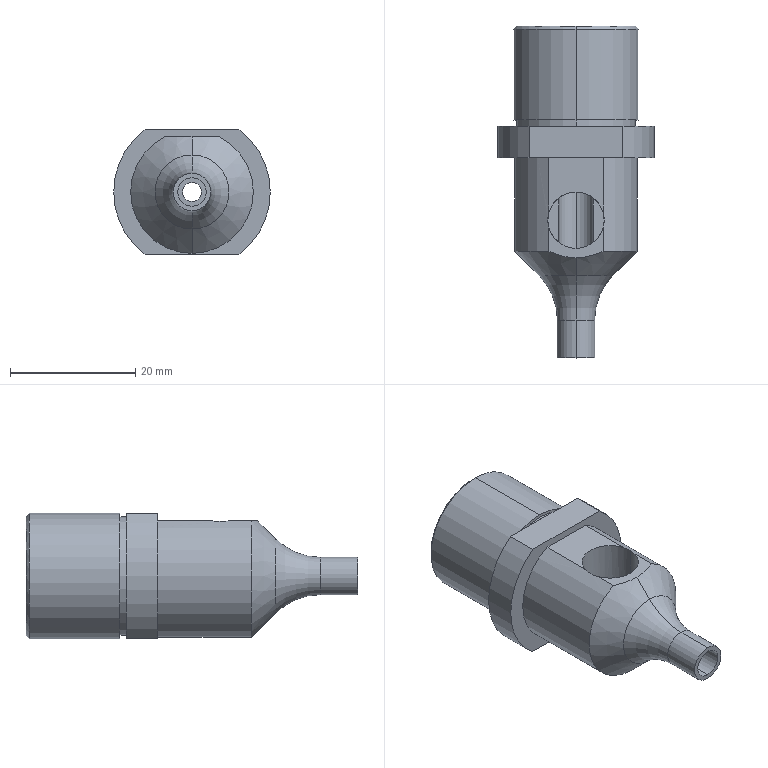Part | SolidWorks | features ICE 7, HoleWzd 4, 3DProfileFeature 2, Chamfer 2, Extrusion 1, Fillet 1, RevCut 1, Revolution 1 | 1 solid | 49 faces | box 25 x 53 x 20 mm | volume 8091 mm3 | cylinder 24 | plane 15 | cone 8 | torus 2 | commonest cylinder face diameters 16 x4 3 x2 4.55 x2 5.5 x2 6 x2 9 x2
STEP:
#1=CARTESIAN_POINT('',(0.,-39.871,-5.929));
#2=VERTEX_POINT('',#1);
#3=CARTESIAN_POINT('',(0.,-39.871,5.929));
#4=VERTEX_POINT('',#3);
#5=CARTESIAN_POINT('',(0.,-39.871,0.));
#6=DIRECTION('',(0.,1.,0.));
#7=DIRECTION('',(0.,0.,-1.));
#8=AXIS2_PLACEMENT_3D('',#5,#6,#7);
#9=CIRCLE('',#8,5.929);
#10=EDGE_CURVE('',#2,#4,#9,.T.);
#11=ORIENTED_EDGE('',*,*,#10,.F.);
#12=CARTESIAN_POINT('',(0.,-46.942,-3.));
#13=VERTEX_POINT('',#12);
#14=CARTESIAN_POINT('',(0.,-46.942,-13.));
#15=DIRECTION('',(1.,0.,0.));
#16=DIRECTION('',(0.,0.,-1.));
#17=AXIS2_PLACEMENT_3D('',#14,#15,#16);
#18=CIRCLE('',#17,10.);
#19=EDGE_CURVE('',#2,#13,#18,.T.);
#20=ORIENTED_EDGE('',*,*,#19,.T.);
#21=CARTESIAN_POINT('',(0.,-46.942,3.));
#22=VERTEX_POINT('',#21);
#23=CARTESIAN_POINT('',(0.,-46.942,0.));
#24=DIRECTION('',(0.,-1.,0.));
#25=DIRECTION('',(0.,0.,1.));
#26=AXIS2_PLACEMENT_3D('',#23,#24,#25);
#27=CIRCLE('',#26,3.);
#28=EDGE_CURVE('',#22,#13,#27,.T.);
#29=ORIENTED_EDGE('',*,*,#28,.F.);
#30=CARTESIAN_POINT('',(0.,-46.942,13.));
#31=DIRECTION('',(-1.,0.,0.));
#32=DIRECTION('',(0.,0.,1.));
#33=AXIS2_PLACEMENT_3D('',#30,#31,#32);
#34=CIRCLE('',#33,10.);
#35=EDGE_CURVE('',#4,#22,#34,.T.);
#36=ORIENTED_EDGE('',*,*,#35,.F.);
#37=EDGE_LOOP('',(#11,#20,#29,#36));
#38=FACE_OUTER_BOUND('',#37,.T.);
#39=CARTESIAN_POINT('',(0.,-46.942,0.));
#40=DIRECTION('',(0.,1.,0.));
#41=DIRECTION('',(0.,0.,1.));
#42=AXIS2_PLACEMENT_3D('',#39,#40,#41);
#43=TOROIDAL_SURFACE('',#42,13.,10.);
#44=ADVANCED_FACE('',(#38),#43,.F.);
#45=CARTESIAN_POINT('',(0.,-48.5,2.275));
#46=VERTEX_POINT('',#45);
#47=CARTESIAN_POINT('',(0.,-48.5,-2.275));
#48=VERTEX_POINT('',#47);
#49=CARTESIAN_POINT('',(0.,-48.5,0.));
#50=DIRECTION('',(0.,-1.,0.));
#51=DIRECTION('',(0.,0.,-1.));
#52=AXIS2_PLACEMENT_3D('',#49,#50,#51);
#53=CIRCLE('',#52,2.275);
#54=EDGE_CURVE('',#46,#48,#53,.T.);
#55=ORIENTED_EDGE('',*,*,#54,.F.);
#56=CARTESIAN_POINT('',(0.,-53.,2.275));
#57=VERTEX_POINT('',#56);
#58=CARTESIAN_POINT('',(0.,-48.5,2.275));
#59=DIRECTION('',(0.,-1.,0.));
#60=VECTOR('',#59,1000.);
#61=LINE('',#58,#60);
#62=EDGE_CURVE('',#46,#57,#61,.T.);
#63=ORIENTED_EDGE('',*,*,#62,.T.);
#64=CARTESIAN_POINT('',(0.,-53.,-2.275));
#65=VERTEX_POINT('',#64);
#66=CARTESIAN_POINT('',(0.,-53.,0.));
#67=DIRECTION('',(0.,-1.,0.));
#68=DIRECTION('',(0.,0.,-1.));
#69=AXIS2_PLACEMENT_3D('',#66,#67,#68);
#70=CIRCLE('',#69,2.275);
#71=EDGE_CURVE('',#57,#65,#70,.T.);
#72=ORIENTED_EDGE('',*,*,#71,.T.);
#73=CARTESIAN_POINT('',(0.,-48.5,-2.275));
#74=DIRECTION('',(0.,-1.,0.));
#75=VECTOR('',#74,1000.);
#76=LINE('',#73,#75);
#77=EDGE_CURVE('',#48,#65,#76,.T.);
#78=ORIENTED_EDGE('',*,*,#77,.F.);
#79=EDGE_LOOP('',(#55,#63,#72,#78));
#80=FACE_OUTER_BOUND('',#79,.T.);
#81=CARTESIAN_POINT('',(0.,-48.5,0.));
#82=DIRECTION('',(0.,-1.,0.));
#83=DIRECTION('',(0.,0.,-1.));
#84=AXIS2_PLACEMENT_3D('',#81,#82,#83);
#85=CYLINDRICAL_SURFACE('',#84,2.275);
#86=ADVANCED_FACE('',(#80),#85,.F.);
#87=CARTESIAN_POINT('',(0.,-43.751,1.5));
#88=VERTEX_POINT('',#87);
#89=CARTESIAN_POINT('',(0.,-43.751,-1.5));
#90=VERTEX_POINT('',#89);
#91=CARTESIAN_POINT('',(0.,-43.751,0.));
#92=DIRECTION('',(0.,-1.,0.));
#93=DIRECTION('',(0.,0.,1.));
#94=AXIS2_PLACEMENT_3D('',#91,#92,#93);
#95=CIRCLE('',#94,1.5);
#96=EDGE_CURVE('',#88,#90,#95,.T.);
#97=ORIENTED_EDGE('',*,*,#96,.T.);
#98=CARTESIAN_POINT('',(0.,-43.,-2.75));
#99=VERTEX_POINT('',#98);
#100=CARTESIAN_POINT('',(0.,-43.,-2.75));
#101=DIRECTION('',(0.,0.515,-0.8572));
#102=VECTOR('',#101,1000.);
#103=LINE('',#100,#102);
#104=EDGE_CURVE('',#90,#99,#103,.T.);
#105=ORIENTED_EDGE('',*,*,#104,.T.);
#106=CARTESIAN_POINT('',(0.,-43.,2.75));
#107=VERTEX_POINT('',#106);
#108=CARTESIAN_POINT('',(0.,-43.,0.));
#109=DIRECTION('',(0.,1.,0.));
#110=DIRECTION('',(0.,0.,1.));
#111=AXIS2_PLACEMENT_3D('',#108,#109,#110);
#112=CIRCLE('',#111,2.75);
#113=EDGE_CURVE('',#99,#107,#112,.T.);
#114=ORIENTED_EDGE('',*,*,#113,.T.);
#115=CARTESIAN_POINT('',(0.,-43.,2.75));
#116=DIRECTION('',(0.,0.515,0.8572));
#117=VECTOR('',#116,1000.);
#118=LINE('',#115,#117);
#119=EDGE_CURVE('',#88,#107,#118,.T.);
#120=ORIENTED_EDGE('',*,*,#119,.F.);
#121=EDGE_LOOP('',(#97,#105,#114,#120));
#122=FACE_OUTER_BOUND('',#121,.T.);
#123=CARTESIAN_POINT('',(0.,-43.,0.));
#124=DIRECTION('',(0.,1.,0.));
#125=DIRECTION('',(0.,0.,1.));
#126=AXIS2_PLACEMENT_3D('',#123,#124,#125);
#127=CONICAL_SURFACE('',#126,2.75,1.03);
#128=ADVANCED_FACE('',(#122),#127,.F.);
#129=ORIENTED_EDGE('',*,*,#113,.F.);
#130=CARTESIAN_POINT('',(0.,-18.,-2.75));
#131=VERTEX_POINT('',#130);
#132=CARTESIAN_POINT('',(0.,-18.,-2.75));
#133=DIRECTION('',(0.,1.,0.));
#134=VECTOR('',#133,1000.);
#135=LINE('',#132,#134);
#136=EDGE_CURVE('',#99,#131,#135,.T.);
#137=ORIENTED_EDGE('',*,*,#136,.T.);
#138=CARTESIAN_POINT('',(0.,-18.,2.75));
#139=VERTEX_POINT('',#138);
#140=CARTESIAN_POINT('',(0.,-18.,0.));
#141=DIRECTION('',(0.,1.,0.));
#142=DIRECTION('',(0.,0.,1.));
#143=AXIS2_PLACEMENT_3D('',#140,#141,#142);
#144=CIRCLE('',#143,2.75);
#145=EDGE_CURVE('',#131,#139,#144,.T.);
#146=ORIENTED_EDGE('',*,*,#145,.T.);
#147=CARTESIAN_POINT('',(0.,-26.5,2.75));
#148=VERTEX_POINT('',#147);
#149=CARTESIAN_POINT('',(0.,-18.,2.75));
#150=DIRECTION('',(0.,1.,0.));
#151=VECTOR('',#150,1000.);
#152=LINE('',#149,#151);
#153=EDGE_CURVE('',#148,#139,#152,.T.);
#154=ORIENTED_EDGE('',*,*,#153,.F.);
#155=CARTESIAN_POINT('',(-2.75,-27.438,0.));
#156=VERTEX_POINT('',#155);
#157=CARTESIAN_POINT('',(-2.75,-27.438,0.));
#158=CARTESIAN_POINT('',(-2.75,-27.438,0.1874));
#159=CARTESIAN_POINT('',(-2.731,-27.423,0.3702));
#160=CARTESIAN_POINT('',(-2.658,-27.369,0.7279));
#161=CARTESIAN_POINT('',(-2.603,-27.329,0.904));
#162=CARTESIAN_POINT('',(-2.395,-27.186,1.398));
#163=CARTESIAN_POINT('',(-2.194,-27.062,1.694));
#164=CARTESIAN_POINT('',(-1.823,-26.884,2.066));
#165=CARTESIAN_POINT('',(-1.686,-26.825,2.18));
#166=CARTESIAN_POINT('',(-1.392,-26.718,2.378));
#167=CARTESIAN_POINT('',(-1.237,-26.67,2.463));
#168=CARTESIAN_POINT('',(-0.9051,-26.589,2.603));
#169=CARTESIAN_POINT('',(-0.7273,-26.555,2.658));
#170=CARTESIAN_POINT('',(-0.3687,-26.511,2.731));
#171=CARTESIAN_POINT('',(-0.1861,-26.5,2.75));
#172=CARTESIAN_POINT('',(0.,-26.5,2.75));
#173=B_SPLINE_CURVE_WITH_KNOTS('',3,(#157,#158,#159,#160,#161,#162,#163,#164,#165,#166,#167,#168,#169,#170,#171,#172),.UNSPECIFIED.,.F.,.F.,(4,2,2,2,2,2,2,4),(0.,0.0005525,0.001105,0.00221,0.002762,0.003315,0.003867,0.00442),.UNSPECIFIED.);
#174=EDGE_CURVE('',#156,#148,#173,.T.);
#175=ORIENTED_EDGE('',*,*,#174,.F.);
#176=CARTESIAN_POINT('',(-2.75,-34.562,0.));
#177=VERTEX_POINT('',#176);
#178=CARTESIAN_POINT('',(-2.75,-18.,0.));
#179=DIRECTION('',(0.,1.,0.));
#180=VECTOR('',#179,1000.);
#181=LINE('',#178,#180);
#182=EDGE_CURVE('',#177,#156,#181,.T.);
#183=ORIENTED_EDGE('',*,*,#182,.F.);
#184=CARTESIAN_POINT('',(0.,-35.5,2.75));
#185=VERTEX_POINT('',#184);
#186=CARTESIAN_POINT('',(0.,-35.5,2.75));
#187=CARTESIAN_POINT('',(-0.1857,-35.5,2.75));
#188=CARTESIAN_POINT('',(-0.3713,-35.488,2.731));
#189=CARTESIAN_POINT('',(-0.7299,-35.444,2.658));
#190=CARTESIAN_POINT('',(-0.9067,-35.411,2.602));
#191=CARTESIAN_POINT('',(-1.405,-35.289,2.391));
#192=CARTESIAN_POINT('',(-1.703,-35.174,2.187));
#193=CARTESIAN_POINT('',(-2.073,-34.997,1.816));
#194=CARTESIAN_POINT('',(-2.185,-34.935,1.679));
#195=CARTESIAN_POINT('',(-2.381,-34.82,1.387));
#196=CARTESIAN_POINT('',(-2.465,-34.766,1.232));
#197=CARTESIAN_POINT('',(-2.603,-34.672,0.9044));
#198=CARTESIAN_POINT('',(-2.658,-34.631,0.7283));
#199=CARTESIAN_POINT('',(-2.731,-34.577,0.3702));
#200=CARTESIAN_POINT('',(-2.75,-34.562,0.1873));
#201=CARTESIAN_POINT('',(-2.75,-34.562,0.));
#202=B_SPLINE_CURVE_WITH_KNOTS('',3,(#186,#187,#188,#189,#190,#191,#192,#193,#194,#195,#196,#197,#198,#199,#200,#201),.UNSPECIFIED.,.F.,.F.,(4,2,2,2,2,2,2,4),(0.00442,0.004971,0.005522,0.006624,0.007176,0.007727,0.008278,0.008829),.UNSPECIFIED.);
#203=EDGE_CURVE('',#185,#177,#202,.T.);
#204=ORIENTED_EDGE('',*,*,#203,.F.);
#205=CARTESIAN_POINT('',(0.,-18.,2.75));
#206=DIRECTION('',(0.,1.,0.));
#207=VECTOR('',#206,1000.);
#208=LINE('',#205,#207);
#209=EDGE_CURVE('',#107,#185,#208,.T.);
#210=ORIENTED_EDGE('',*,*,#209,.F.);
#211=EDGE_LOOP('',(#129,#137,#146,#154,#175,#183,#204,#210));
#212=FACE_OUTER_BOUND('',#211,.T.);
#213=CARTESIAN_POINT('',(0.,-18.,0.));
#214=DIRECTION('',(0.,1.,0.));
#215=DIRECTION('',(0.,0.,1.));
#216=AXIS2_PLACEMENT_3D('',#213,#214,#215);
#217=CYLINDRICAL_SURFACE('',#216,2.75);
#218=ADVANCED_FACE('',(#212),#217,.F.);
#219=CARTESIAN_POINT('',(0.,-53.,3.));
#220=VERTEX_POINT('',#219);
#221=CARTESIAN_POINT('',(0.,-53.,-3.));
#222=VERTEX_POINT('',#221);
#223=CARTESIAN_POINT('',(0.,-53.,0.));
#224=DIRECTION('',(0.,1.,0.));
#225=DIRECTION('',(0.,0.,1.));
#226=AXIS2_PLACEMENT_3D('',#223,#224,#225);
#227=CIRCLE('',#226,3.);
#228=EDGE_CURVE('',#220,#222,#227,.T.);
#229=ORIENTED_EDGE('',*,*,#228,.T.);
#230=CARTESIAN_POINT('',(0.,2.516,-3.));
#231=DIRECTION('',(0.,1.,0.));
#232=VECTOR('',#231,1000.);
#233=LINE('',#230,#232);
#234=EDGE_CURVE('',#222,#13,#233,.T.);
#235=ORIENTED_EDGE('',*,*,#234,.T.);
#236=CARTESIAN_POINT('',(0.,-46.942,0.));
#237=DIRECTION('',(0.,-1.,0.));
#238=DIRECTION('',(0.,0.,1.));
#239=AXIS2_PLACEMENT_3D('',#236,#237,#238);
#240=CIRCLE('',#239,3.);
#241=EDGE_CURVE('',#13,#22,#240,.T.);
#242=ORIENTED_EDGE('',*,*,#241,.T.);
#243=CARTESIAN_POINT('',(0.,2.516,3.));
#244=DIRECTION('',(0.,1.,0.));
#245=VECTOR('',#244,1000.);
#246=LINE('',#243,#245);
#247=EDGE_CURVE('',#220,#22,#246,.T.);
#248=ORIENTED_EDGE('',*,*,#247,.F.);
#249=EDGE_LOOP('',(#229,#235,#242,#248));
#250=FACE_OUTER_BOUND('',#249,.T.);
#251=CARTESIAN_POINT('',(0.,2.516,0.));
#252=DIRECTION('',(0.,1.,0.));
#253=DIRECTION('',(0.,0.,1.));
#254=AXIS2_PLACEMENT_3D('',#251,#252,#253);
#255=CYLINDRICAL_SURFACE('',#254,3.);
#256=ADVANCED_FACE('',(#250),#255,.T.);
#257=CARTESIAN_POINT('',(0.,-39.871,0.));
#258=DIRECTION('',(0.,1.,0.));
#259=DIRECTION('',(0.,0.,-1.));
#260=AXIS2_PLACEMENT_3D('',#257,#258,#259);
#261=CIRCLE('',#260,5.929);
#262=EDGE_CURVE('',#4,#2,#261,.T.);
#263=ORIENTED_EDGE('',*,*,#262,.T.);
#264=CARTESIAN_POINT('',(0.,-36.,-9.8));
#265=VERTEX_POINT('',#264);
#266=CARTESIAN_POINT('',(0.,-38.,-7.8));
#267=DIRECTION('',(0.,0.7071,-0.7071));
#268=VECTOR('',#267,1000.);
#269=LINE('',#266,#268);
#270=EDGE_CURVE('',#2,#265,#269,.T.);
#271=ORIENTED_EDGE('',*,*,#270,.T.);
#272=CARTESIAN_POINT('',(4.313,-36.,8.8));
#273=VERTEX_POINT('',#272);
#274=CARTESIAN_POINT('',(0.,-36.,0.));
#275=DIRECTION('',(0.,1.,0.));
#276=DIRECTION('',(0.,0.,1.));
#277=AXIS2_PLACEMENT_3D('',#274,#275,#276);
#278=CIRCLE('',#277,9.8);
#279=EDGE_CURVE('',#273,#265,#278,.T.);
#280=ORIENTED_EDGE('',*,*,#279,.F.);
#281=CARTESIAN_POINT('',(0.,-37.,8.8));
#282=VERTEX_POINT('',#281);
#283=CARTESIAN_POINT('',(0.,-37.,8.8));
#284=CARTESIAN_POINT('',(0.7477,-37.,8.8));
#285=CARTESIAN_POINT('',(1.48,-36.904,8.8));
#286=CARTESIAN_POINT('',(2.921,-36.554,8.8));
#287=CARTESIAN_POINT('',(3.634,-36.299,8.8));
#288=CARTESIAN_POINT('',(4.313,-36.,8.8));
#289=B_SPLINE_CURVE_WITH_KNOTS('',3,(#283,#284,#285,#286,#287,#288),.UNSPECIFIED.,.F.,.F.,(4,2,4),(0.00443,0.006647,0.008864),.UNSPECIFIED.);
#290=EDGE_CURVE('',#282,#273,#289,.T.);
#291=ORIENTED_EDGE('',*,*,#290,.F.);
#292=CARTESIAN_POINT('',(0.,-38.,7.8));
#293=DIRECTION('',(0.,0.7071,0.7071));
#294=VECTOR('',#293,1000.);
#295=LINE('',#292,#294);
#296=EDGE_CURVE('',#4,#282,#295,.T.);
#297=ORIENTED_EDGE('',*,*,#296,.F.);
#298=EDGE_LOOP('',(#263,#271,#280,#291,#297));
#299=FACE_OUTER_BOUND('',#298,.T.);
#300=CARTESIAN_POINT('',(0.,-38.,0.));
#301=DIRECTION('',(0.,1.,0.));
#302=DIRECTION('',(0.,0.,1.));
#303=AXIS2_PLACEMENT_3D('',#300,#301,#302);
#304=CONICAL_SURFACE('',#303,7.8,0.7854);
#305=ADVANCED_FACE('',(#299),#304,.T.);
#306=CARTESIAN_POINT('',(0.,-15.,9.5));
#307=VERTEX_POINT('',#306);
#308=CARTESIAN_POINT('',(0.,-15.,-9.5));
#309=VERTEX_POINT('',#308);
#310=CARTESIAN_POINT('',(0.,-15.,0.));
#311=DIRECTION('',(0.,1.,0.));
#312=DIRECTION('',(0.,0.,1.));
#313=AXIS2_PLACEMENT_3D('',#310,#311,#312);
#314=CIRCLE('',#313,9.5);
#315=EDGE_CURVE('',#307,#309,#314,.T.);
#316=ORIENTED_EDGE('',*,*,#315,.F.);
#317=CARTESIAN_POINT('',(0.,-16.,9.5));
#318=VERTEX_POINT('',#317);
#319=CARTESIAN_POINT('',(0.,-15.,9.5));
#320=DIRECTION('',(0.,-1.,0.));
#321=VECTOR('',#320,1000.);
#322=LINE('',#319,#321);
#323=EDGE_CURVE('',#307,#318,#322,.T.);
#324=ORIENTED_EDGE('',*,*,#323,.T.);
#325=CARTESIAN_POINT('',(0.,-16.,-9.5));
#326=VERTEX_POINT('',#325);
#327=CARTESIAN_POINT('',(0.,-16.,0.));
#328=DIRECTION('',(0.,1.,0.));
#329=DIRECTION('',(0.,0.,1.));
#330=AXIS2_PLACEMENT_3D('',#327,#328,#329);
#331=CIRCLE('',#330,9.5);
#332=EDGE_CURVE('',#318,#326,#331,.T.);
#333=ORIENTED_EDGE('',*,*,#332,.T.);
#334=CARTESIAN_POINT('',(0.,-15.,-9.5));
#335=DIRECTION('',(0.,-1.,0.));
#336=VECTOR('',#335,1000.);
#337=LINE('',#334,#336);
#338=EDGE_CURVE('',#309,#326,#337,.T.);
#339=ORIENTED_EDGE('',*,*,#338,.F.);
#340=EDGE_LOOP('',(#316,#324,#333,#339));
#341=FACE_OUTER_BOUND('',#340,.T.);
#342=CARTESIAN_POINT('',(0.,-15.,0.));
#343=DIRECTION('',(0.,-1.,0.));
#344=DIRECTION('',(0.,0.,-1.));
#345=AXIS2_PLACEMENT_3D('',#342,#343,#344);
#346=CYLINDRICAL_SURFACE('',#345,9.5);
#347=ADVANCED_FACE('',(#341),#346,.T.);
#348=CARTESIAN_POINT('',(0.,-0.5,-8.));
#349=VERTEX_POINT('',#348);
#350=CARTESIAN_POINT('',(0.,-0.5,8.));
#351=VERTEX_POINT('',#350);
#352=CARTESIAN_POINT('',(0.,-0.5,0.));
#353=DIRECTION('',(0.,1.,0.));
#354=DIRECTION('',(0.,0.,1.));
#355=AXIS2_PLACEMENT_3D('',#352,#353,#354);
#356=CIRCLE('',#355,8.);
#357=EDGE_CURVE('',#349,#351,#356,.T.);
#358=ORIENTED_EDGE('',*,*,#357,.F.);
#359=CARTESIAN_POINT('',(0.,0.,-8.5));
#360=VERTEX_POINT('',#359);
#361=CARTESIAN_POINT('',(0.,-0.5,-8.));
#362=DIRECTION('',(0.,0.7071,-0.7071));
#363=VECTOR('',#362,1000.);
#364=LINE('',#361,#363);
#365=EDGE_CURVE('',#349,#360,#364,.T.);
#366=ORIENTED_EDGE('',*,*,#365,.T.);
#367=CARTESIAN_POINT('',(0.,0.,8.5));
#368=VERTEX_POINT('',#367);
#369=CARTESIAN_POINT('',(0.,0.,0.));
#370=DIRECTION('',(0.,-1.,0.));
#371=DIRECTION('',(0.,0.,1.));
#372=AXIS2_PLACEMENT_3D('',#369,#370,#371);
#373=CIRCLE('',#372,8.5);
#374=EDGE_CURVE('',#368,#360,#373,.T.);
#375=ORIENTED_EDGE('',*,*,#374,.F.);
#376=CARTESIAN_POINT('',(0.,-0.5,8.));
#377=DIRECTION('',(0.,0.7071,0.7071));
#378=VECTOR('',#377,1000.);
#379=LINE('',#376,#378);
#380=EDGE_CURVE('',#351,#368,#379,.T.);
#381=ORIENTED_EDGE('',*,*,#380,.F.);
#382=EDGE_LOOP('',(#358,#366,#375,#381));
#383=FACE_OUTER_BOUND('',#382,.T.);
#384=CARTESIAN_POINT('',(0.,-0.5,0.));
#385=DIRECTION('',(0.,1.,0.));
#386=DIRECTION('',(0.,0.,1.));
#387=AXIS2_PLACEMENT_3D('',#384,#385,#386);
#388=CONICAL_SURFACE('',#387,8.,0.7854);
#389=ADVANCED_FACE('',(#383),#388,.F.);
#390=CARTESIAN_POINT('',(0.,0.,9.5));
#391=VERTEX_POINT('',#390);
#392=CARTESIAN_POINT('',(0.,0.,-9.5));
#393=VERTEX_POINT('',#392);
#394=CARTESIAN_POINT('',(0.,0.,0.));
#395=DIRECTION('',(0.,1.,0.));
#396=DIRECTION('',(0.,0.,1.));
#397=AXIS2_PLACEMENT_3D('',#394,#395,#396);
#398=CIRCLE('',#397,9.5);
#399=EDGE_CURVE('',#391,#393,#398,.T.);
#400=ORIENTED_EDGE('',*,*,#399,.F.);
#401=CARTESIAN_POINT('',(0.,-0.5,10.));
#402=VERTEX_POINT('',#401);
#403=CARTESIAN_POINT('',(0.,0.,9.5));
#404=DIRECTION('',(0.,-0.7071,0.7071));
#405=VECTOR('',#404,1000.);
#406=LINE('',#403,#405);
#407=EDGE_CURVE('',#391,#402,#406,.T.);
#408=ORIENTED_EDGE('',*,*,#407,.T.);
#409=CARTESIAN_POINT('',(0.,-0.5,-10.));
#410=VERTEX_POINT('',#409);
#411=CARTESIAN_POINT('',(0.,-0.5,0.));
#412=DIRECTION('',(0.,-1.,0.));
#413=DIRECTION('',(0.,0.,1.));
#414=AXIS2_PLACEMENT_3D('',#411,#412,#413);
#415=CIRCLE('',#414,10.);
#416=EDGE_CURVE('',#410,#402,#415,.T.);
#417=ORIENTED_EDGE('',*,*,#416,.F.);
#418=CARTESIAN_POINT('',(0.,0.,-9.5));
#419=DIRECTION('',(0.,-0.7071,-0.7071));
#420=VECTOR('',#419,1000.);
#421=LINE('',#418,#420);
#422=EDGE_CURVE('',#393,#410,#421,.T.);
#423=ORIENTED_EDGE('',*,*,#422,.F.);
#424=EDGE_LOOP('',(#400,#408,#417,#423));
#425=FACE_OUTER_BOUND('',#424,.T.);
#426=CARTESIAN_POINT('',(0.,0.,0.));
#427=DIRECTION('',(0.,-1.,0.));
#428=DIRECTION('',(0.,0.,-1.));
#429=AXIS2_PLACEMENT_3D('',#426,#427,#428);
#430=CONICAL_SURFACE('',#429,9.5,0.7854);
#431=ADVANCED_FACE('',(#425),#430,.T.);
#432=CARTESIAN_POINT('',(-4.313,-21.,8.8));
#433=VERTEX_POINT('',#432);
#434=CARTESIAN_POINT('',(0.,-21.,-9.8));
#435=VERTEX_POINT('',#434);
#436=CARTESIAN_POINT('',(0.,-21.,0.));
#437=DIRECTION('',(0.,-1.,0.));
#438=DIRECTION('',(0.,0.,1.));
#439=AXIS2_PLACEMENT_3D('',#436,#437,#438);
#440=CIRCLE('',#439,9.8);
#441=EDGE_CURVE('',#433,#435,#440,.T.);
#442=ORIENTED_EDGE('',*,*,#441,.T.);
#443=CARTESIAN_POINT('',(0.,7.284,-9.8));
#444=DIRECTION('',(0.,-1.,0.));
#445=VECTOR('',#444,1000.);
#446=LINE('',#443,#445);
#447=EDGE_CURVE('',#435,#265,#446,.T.);
#448=ORIENTED_EDGE('',*,*,#447,.T.);
#449=CARTESIAN_POINT('',(-4.313,-36.,8.8));
#450=VERTEX_POINT('',#449);
#451=CARTESIAN_POINT('',(0.,-36.,0.));
#452=DIRECTION('',(0.,1.,0.));
#453=DIRECTION('',(0.,0.,1.));
#454=AXIS2_PLACEMENT_3D('',#451,#452,#453);
#455=CIRCLE('',#454,9.8);
#456=EDGE_CURVE('',#265,#450,#455,.T.);
#457=ORIENTED_EDGE('',*,*,#456,.T.);
#458=CARTESIAN_POINT('',(-4.313,-32.285,8.8));
#459=VERTEX_POINT('',#458);
#460=CARTESIAN_POINT('',(-4.313,7.284,8.8));
#461=DIRECTION('',(0.,-1.,0.));
#462=VECTOR('',#461,1000.);
#463=LINE('',#460,#462);
#464=EDGE_CURVE('',#459,#450,#463,.T.);
#465=ORIENTED_EDGE('',*,*,#464,.F.);
#466=CARTESIAN_POINT('',(-4.5,-31.,8.706));
#467=VERTEX_POINT('',#466);
#468=CARTESIAN_POINT('',(-4.313,-32.285,8.8));
#469=CARTESIAN_POINT('',(-4.374,-32.08,8.77));
#470=CARTESIAN_POINT('',(-4.42,-31.87,8.746));
#471=CARTESIAN_POINT('',(-4.484,-31.44,8.714));
#472=CARTESIAN_POINT('',(-4.5,-31.22,8.706));
#473=CARTESIAN_POINT('',(-4.5,-31.,8.706));
#474=B_SPLINE_CURVE_WITH_KNOTS('',3,(#468,#469,#470,#471,#472,#473),.UNSPECIFIED.,.F.,.F.,(4,2,4),(0.02723,0.02788,0.02852),.UNSPECIFIED.);
#475=EDGE_CURVE('',#459,#467,#474,.T.);
#476=ORIENTED_EDGE('',*,*,#475,.T.);
#477=CARTESIAN_POINT('',(-4.313,-29.715,8.8));
#478=VERTEX_POINT('',#477);
#479=CARTESIAN_POINT('',(-4.5,-31.,8.706));
#480=CARTESIAN_POINT('',(-4.5,-30.78,8.706));
#481=CARTESIAN_POINT('',(-4.484,-30.563,8.714));
#482=CARTESIAN_POINT('',(-4.421,-30.135,8.746));
#483=CARTESIAN_POINT('',(-4.375,-29.923,8.77));
#484=CARTESIAN_POINT('',(-4.313,-29.715,8.8));
#485=B_SPLINE_CURVE_WITH_KNOTS('',3,(#479,#480,#481,#482,#483,#484),.UNSPECIFIED.,.F.,.F.,(4,2,4),(0.,0.0006507,0.001301),.UNSPECIFIED.);
#486=EDGE_CURVE('',#467,#478,#485,.T.);
#487=ORIENTED_EDGE('',*,*,#486,.T.);
#488=CARTESIAN_POINT('',(-4.313,7.284,8.8));
#489=DIRECTION('',(0.,-1.,0.));
#490=VECTOR('',#489,1000.);
#491=LINE('',#488,#490);
#492=EDGE_CURVE('',#433,#478,#491,.T.);
#493=ORIENTED_EDGE('',*,*,#492,.F.);
#494=EDGE_LOOP('',(#442,#448,#457,#465,#476,#487,#493));
#495=FACE_OUTER_BOUND('',#494,.T.);
#496=CARTESIAN_POINT('',(0.,7.284,0.));
#497=DIRECTION('',(0.,-1.,0.));
#498=DIRECTION('',(0.,0.,-1.));
#499=AXIS2_PLACEMENT_3D('',#496,#497,#498);
#500=CYLINDRICAL_SURFACE('',#499,9.8);
#501=ADVANCED_FACE('',(#495),#500,.T.);
#502=CARTESIAN_POINT('',(0.,-1.8,8.5));
#503=VERTEX_POINT('',#502);
#504=CARTESIAN_POINT('',(0.,-1.8,-8.5));
#505=VERTEX_POINT('',#504);
#506=CARTESIAN_POINT('',(0.,-1.8,0.));
#507=DIRECTION('',(0.,-1.,0.));
#508=DIRECTION('',(0.,0.,-1.));
#509=AXIS2_PLACEMENT_3D('',#506,#507,#508);
#510=CIRCLE('',#509,8.5);
#511=EDGE_CURVE('',#503,#505,#510,.T.);
#512=ORIENTED_EDGE('',*,*,#511,.F.);
#513=CARTESIAN_POINT('',(0.,-3.,8.5));
#514=VERTEX_POINT('',#513);
#515=CARTESIAN_POINT('',(0.,-38.,8.5));
#516=DIRECTION('',(0.,-1.,0.));
#517=VECTOR('',#516,1000.);
#518=LINE('',#515,#517);
#519=EDGE_CURVE('',#503,#514,#518,.T.);
#520=ORIENTED_EDGE('',*,*,#519,.T.);
#521=CARTESIAN_POINT('',(0.,-3.,-8.5));
#522=VERTEX_POINT('',#521);
#523=CARTESIAN_POINT('',(0.,-3.,0.));
#524=DIRECTION('',(0.,-1.,0.));
#525=DIRECTION('',(0.,0.,-1.));
#526=AXIS2_PLACEMENT_3D('',#523,#524,#525);
#527=CIRCLE('',#526,8.5);
#528=EDGE_CURVE('',#514,#522,#527,.T.);
#529=ORIENTED_EDGE('',*,*,#528,.T.);
#530=CARTESIAN_POINT('',(0.,-38.,-8.5));
#531=DIRECTION('',(0.,-1.,0.));
#532=VECTOR('',#531,1000.);
#533=LINE('',#530,#532);
#534=EDGE_CURVE('',#505,#522,#533,.T.);
#535=ORIENTED_EDGE('',*,*,#534,.F.);
#536=EDGE_LOOP('',(#512,#520,#529,#535));
#537=FACE_OUTER_BOUND('',#536,.T.);
#538=CARTESIAN_POINT('',(0.,-38.,0.));
#539=DIRECTION('',(0.,-1.,0.));
#540=DIRECTION('',(0.,0.,-1.));
#541=AXIS2_PLACEMENT_3D('',#538,#539,#540);
#542=CYLINDRICAL_SURFACE('',#541,8.5);
#543=ADVANCED_FACE('',(#537),#542,.F.);
#544=CARTESIAN_POINT('',(0.,-18.,-8.));
#545=VERTEX_POINT('',#544);
#546=CARTESIAN_POINT('',(0.,-18.,8.));
#547=VERTEX_POINT('',#546);
#548=CARTESIAN_POINT('',(0.,-18.,0.));
#549=DIRECTION('',(0.,1.,0.));
#550=DIRECTION('',(0.,0.,1.));
#551=AXIS2_PLACEMENT_3D('',#548,#549,#550);
#552=CIRCLE('',#551,8.);
#553=EDGE_CURVE('',#545,#547,#552,.T.);
#554=ORIENTED_EDGE('',*,*,#553,.F.);
#555=CARTESIAN_POINT('',(0.,-3.,-8.));
#556=VERTEX_POINT('',#555);
#557=CARTESIAN_POINT('',(0.,-18.,-8.));
#558=DIRECTION('',(0.,1.,0.));
#559=VECTOR('',#558,1000.);
#560=LINE('',#557,#559);
#561=EDGE_CURVE('',#545,#556,#560,.T.);
#562=ORIENTED_EDGE('',*,*,#561,.T.);
#563=CARTESIAN_POINT('',(0.,-3.,8.));
#564=VERTEX_POINT('',#563);
#565=CARTESIAN_POINT('',(0.,-3.,0.));
#566=DIRECTION('',(0.,1.,0.));
#567=DIRECTION('',(0.,0.,-1.));
#568=AXIS2_PLACEMENT_3D('',#565,#566,#567);
#569=CIRCLE('',#568,8.);
#570=EDGE_CURVE('',#556,#564,#569,.T.);
#571=ORIENTED_EDGE('',*,*,#570,.T.);
#572=CARTESIAN_POINT('',(0.,-18.,8.));
#573=DIRECTION('',(0.,1.,0.));
#574=VECTOR('',#573,1000.);
#575=LINE('',#572,#574);
#576=EDGE_CURVE('',#547,#564,#575,.T.);
#577=ORIENTED_EDGE('',*,*,#576,.F.);
#578=EDGE_LOOP('',(#554,#562,#571,#577));
#579=FACE_OUTER_BOUND('',#578,.T.);
#580=CARTESIAN_POINT('',(0.,-18.,0.));
#581=DIRECTION('',(0.,1.,0.));
#582=DIRECTION('',(0.,0.,1.));
#583=AXIS2_PLACEMENT_3D('',#580,#581,#582);
#584=CYLINDRICAL_SURFACE('',#583,8.);
#585=ADVANCED_FACE('',(#579),#584,.F.);
#586=CARTESIAN_POINT('',(0.,-15.,-10.));
#587=VERTEX_POINT('',#586);
#588=CARTESIAN_POINT('',(0.,-15.,10.));
#589=VERTEX_POINT('',#588);
#590=CARTESIAN_POINT('',(0.,-15.,0.));
#591=DIRECTION('',(0.,-1.,0.));
#592=DIRECTION('',(0.,0.,1.));
#593=AXIS2_PLACEMENT_3D('',#590,#591,#592);
#594=CIRCLE('',#593,10.);
#595=EDGE_CURVE('',#587,#589,#594,.T.);
#596=ORIENTED_EDGE('',*,*,#595,.F.);
#597=CARTESIAN_POINT('',(0.,-38.,-10.));
#598=DIRECTION('',(0.,1.,0.));
#599=VECTOR('',#598,1000.);
#600=LINE('',#597,#599);
#601=EDGE_CURVE('',#587,#410,#600,.T.);
#602=ORIENTED_EDGE('',*,*,#601,.T.);
#603=ORIENTED_EDGE('',*,*,#416,.T.);
#604=CARTESIAN_POINT('',(0.,-38.,10.));
#605=DIRECTION('',(0.,1.,0.));
#606=VECTOR('',#605,1000.);
#607=LINE('',#604,#606);
#608=EDGE_CURVE('',#589,#402,#607,.T.);
#609=ORIENTED_EDGE('',*,*,#608,.F.);
#610=EDGE_LOOP('',(#596,#602,#603,#609));
#611=FACE_OUTER_BOUND('',#610,.T.);
#612=CARTESIAN_POINT('',(0.,-38.,0.));
#613=DIRECTION('',(0.,1.,0.));
#614=DIRECTION('',(0.,0.,1.));
#615=AXIS2_PLACEMENT_3D('',#612,#613,#614);
#616=CYLINDRICAL_SURFACE('',#615,10.);
#617=ADVANCED_FACE('',(#611),#616,.T.);
#618=CARTESIAN_POINT('',(0.,-1.8,8.));
#619=VERTEX_POINT('',#618);
#620=CARTESIAN_POINT('',(0.,-1.8,-8.));
#621=VERTEX_POINT('',#620);
#622=CARTESIAN_POINT('',(0.,-1.8,0.));
#623=DIRECTION('',(0.,-1.,0.));
#624=DIRECTION('',(0.,0.,1.));
#625=AXIS2_PLACEMENT_3D('',#622,#623,#624);
#626=CIRCLE('',#625,8.);
#627=EDGE_CURVE('',#619,#621,#626,.T.);
#628=ORIENTED_EDGE('',*,*,#627,.T.);
#629=CARTESIAN_POINT('',(0.,-18.,-8.));
#630=DIRECTION('',(0.,1.,0.));
#631=VECTOR('',#630,1000.);
#632=LINE('',#629,#631);
#633=EDGE_CURVE('',#621,#349,#632,.T.);
#634=ORIENTED_EDGE('',*,*,#633,.T.);
#635=ORIENTED_EDGE('',*,*,#357,.T.);
#636=CARTESIAN_POINT('',(0.,-18.,8.));
#637=DIRECTION('',(0.,1.,0.));
#638=VECTOR('',#637,1000.);
#639=LINE('',#636,#638);
#640=EDGE_CURVE('',#619,#351,#639,.T.);
#641=ORIENTED_EDGE('',*,*,#640,.F.);
#642=EDGE_LOOP('',(#628,#634,#635,#641));
#643=FACE_OUTER_BOUND('',#642,.T.);
#644=CARTESIAN_POINT('',(0.,-18.,0.));
#645=DIRECTION('',(0.,1.,0.));
#646=DIRECTION('',(0.,0.,1.));
#647=AXIS2_PLACEMENT_3D('',#644,#645,#646);
#648=CYLINDRICAL_SURFACE('',#647,8.);
#649=ADVANCED_FACE('',(#643),#648,.F.);
#650=CARTESIAN_POINT('',(4.5,-31.,8.706));
#651=VERTEX_POINT('',#650);
#652=CARTESIAN_POINT('',(4.313,-32.285,8.8));
#653=VERTEX_POINT('',#652);
#654=CARTESIAN_POINT('',(4.5,-31.,8.706));
#655=CARTESIAN_POINT('',(4.5,-31.216,8.706));
#656=CARTESIAN_POINT('',(4.484,-31.435,8.714));
#657=CARTESIAN_POINT('',(4.421,-31.868,8.746));
#658=CARTESIAN_POINT('',(4.374,-32.079,8.77));
#659=CARTESIAN_POINT('',(4.313,-32.285,8.8));
#660=B_SPLINE_CURVE_WITH_KNOTS('',3,(#654,#655,#656,#657,#658,#659),.UNSPECIFIED.,.F.,.F.,(4,2,4),(0.01427,0.01492,0.01557),.UNSPECIFIED.);
#661=EDGE_CURVE('',#651,#653,#660,.T.);
#662=ORIENTED_EDGE('',*,*,#661,.F.);
#663=CARTESIAN_POINT('',(4.5,-31.,0.));
#664=VERTEX_POINT('',#663);
#665=CARTESIAN_POINT('',(4.5,-31.,0.));
#666=DIRECTION('',(0.,0.,-1.));
#667=VECTOR('',#666,1000.);
#668=LINE('',#665,#667);
#669=EDGE_CURVE('',#651,#664,#668,.T.);
#670=ORIENTED_EDGE('',*,*,#669,.T.);
#671=CARTESIAN_POINT('',(2.75,-34.562,0.));
#672=VERTEX_POINT('',#671);
#673=CARTESIAN_POINT('',(0.,-31.,0.));
#674=DIRECTION('',(0.,0.,-1.));
#675=DIRECTION('',(-1.,0.,0.));
#676=AXIS2_PLACEMENT_3D('',#673,#674,#675);
#677=CIRCLE('',#676,4.5);
#678=EDGE_CURVE('',#664,#672,#677,.T.);
#679=ORIENTED_EDGE('',*,*,#678,.T.);
#680=CARTESIAN_POINT('',(2.75,-34.562,0.));
#681=CARTESIAN_POINT('',(2.75,-34.562,0.1874));
#682=CARTESIAN_POINT('',(2.731,-34.577,0.3702));
#683=CARTESIAN_POINT('',(2.658,-34.631,0.7279));
#684=CARTESIAN_POINT('',(2.603,-34.671,0.904));
#685=CARTESIAN_POINT('',(2.395,-34.814,1.398));
#686=CARTESIAN_POINT('',(2.194,-34.938,1.694));
#687=CARTESIAN_POINT('',(1.823,-35.116,2.066));
#688=CARTESIAN_POINT('',(1.686,-35.175,2.18));
#689=CARTESIAN_POINT('',(1.392,-35.282,2.378));
#690=CARTESIAN_POINT('',(1.237,-35.33,2.463));
#691=CARTESIAN_POINT('',(0.9051,-35.411,2.603));
#692=CARTESIAN_POINT('',(0.7273,-35.445,2.658));
#693=CARTESIAN_POINT('',(0.3687,-35.489,2.731));
#694=CARTESIAN_POINT('',(0.1861,-35.5,2.75));
#695=CARTESIAN_POINT('',(0.,-35.5,2.75));
#696=B_SPLINE_CURVE_WITH_KNOTS('',3,(#680,#681,#682,#683,#684,#685,#686,#687,#688,#689,#690,#691,#692,#693,#694,#695),.UNSPECIFIED.,.F.,.F.,(4,2,2,2,2,2,2,4),(0.,0.0005525,0.001105,0.00221,0.002762,0.003315,0.003867,0.00442),.UNSPECIFIED.);
#697=EDGE_CURVE('',#672,#185,#696,.T.);
#698=ORIENTED_EDGE('',*,*,#697,.T.);
#699=ORIENTED_EDGE('',*,*,#203,.T.);
#700=CARTESIAN_POINT('',(-4.5,-31.,0.));
#701=VERTEX_POINT('',#700);
#702=CARTESIAN_POINT('',(0.,-31.,0.));
#703=DIRECTION('',(0.,0.,-1.));
#704=DIRECTION('',(-1.,0.,0.));
#705=AXIS2_PLACEMENT_3D('',#702,#703,#704);
#706=CIRCLE('',#705,4.5);
#707=EDGE_CURVE('',#177,#701,#706,.T.);
#708=ORIENTED_EDGE('',*,*,#707,.T.);
#709=CARTESIAN_POINT('',(-4.5,-31.,0.));
#710=DIRECTION('',(0.,0.,-1.));
#711=VECTOR('',#710,1000.);
#712=LINE('',#709,#711);
#713=EDGE_CURVE('',#467,#701,#712,.T.);
#714=ORIENTED_EDGE('',*,*,#713,.F.);
#715=ORIENTED_EDGE('',*,*,#475,.F.);
#716=CARTESIAN_POINT('',(0.,-31.,8.8));
#717=DIRECTION('',(0.,0.,1.));
#718=DIRECTION('',(0.,1.,0.));
#719=AXIS2_PLACEMENT_3D('',#716,#717,#718);
#720=CIRCLE('',#719,4.5);
#721=EDGE_CURVE('',#459,#653,#720,.T.);
#722=ORIENTED_EDGE('',*,*,#721,.T.);
#723=EDGE_LOOP('',(#662,#670,#679,#698,#699,#708,#714,#715,#722));
#724=FACE_OUTER_BOUND('',#723,.T.);
#725=CARTESIAN_POINT('',(0.,-31.,0.));
#726=DIRECTION('',(0.,0.,-1.));
#727=DIRECTION('',(-1.,0.,0.));
#728=AXIS2_PLACEMENT_3D('',#725,#726,#727);
#729=CYLINDRICAL_SURFACE('',#728,4.5);
#730=ADVANCED_FACE('',(#724),#729,.F.);
#731=ORIENTED_EDGE('',*,*,#96,.F.);
#732=CARTESIAN_POINT('',(0.,-48.5,1.5));
#733=VERTEX_POINT('',#732);
#734=CARTESIAN_POINT('',(0.,-53.,1.5));
#735=DIRECTION('',(0.,-1.,0.));
#736=VECTOR('',#735,1000.);
#737=LINE('',#734,#736);
#738=EDGE_CURVE('',#88,#733,#737,.T.);
#739=ORIENTED_EDGE('',*,*,#738,.T.);
#740=CARTESIAN_POINT('',(0.,-48.5,-1.5));
#741=VERTEX_POINT('',#740);
#742=CARTESIAN_POINT('',(0.,-48.5,0.));
#743=DIRECTION('',(0.,1.,0.));
#744=DIRECTION('',(0.,0.,-1.));
#745=AXIS2_PLACEMENT_3D('',#742,#743,#744);
#746=CIRCLE('',#745,1.5);
#747=EDGE_CURVE('',#741,#733,#746,.T.);
#748=ORIENTED_EDGE('',*,*,#747,.F.);
#749=CARTESIAN_POINT('',(0.,-53.,-1.5));
#750=DIRECTION('',(0.,-1.,0.));
#751=VECTOR('',#750,1000.);
#752=LINE('',#749,#751);
#753=EDGE_CURVE('',#90,#741,#752,.T.);
#754=ORIENTED_EDGE('',*,*,#753,.F.);
#755=EDGE_LOOP('',(#731,#739,#748,#754));
#756=FACE_OUTER_BOUND('',#755,.T.);
#757=CARTESIAN_POINT('',(0.,-53.,0.));
#758=DIRECTION('',(0.,-1.,0.));
#759=DIRECTION('',(0.,0.,-1.));
#760=AXIS2_PLACEMENT_3D('',#757,#758,#759);
#761=CYLINDRICAL_SURFACE('',#760,1.5);
#762=ADVANCED_FACE('',(#756),#761,.F.);
#763=ORIENTED_EDGE('',*,*,#738,.F.);
#764=CARTESIAN_POINT('',(0.,-43.751,0.));
#765=DIRECTION('',(0.,-1.,0.));
#766=DIRECTION('',(0.,0.,1.));
#767=AXIS2_PLACEMENT_3D('',#764,#765,#766);
#768=CIRCLE('',#767,1.5);
#769=EDGE_CURVE('',#90,#88,#768,.T.);
#770=ORIENTED_EDGE('',*,*,#769,.F.);
#771=ORIENTED_EDGE('',*,*,#753,.T.);
#772=CARTESIAN_POINT('',(0.,-48.5,0.));
#773=DIRECTION('',(0.,1.,0.));
#774=DIRECTION('',(0.,0.,-1.));
#775=AXIS2_PLACEMENT_3D('',#772,#773,#774);
#776=CIRCLE('',#775,1.5);
#777=EDGE_CURVE('',#733,#741,#776,.T.);
#778=ORIENTED_EDGE('',*,*,#777,.F.);
#779=EDGE_LOOP('',(#763,#770,#771,#778));
#780=FACE_OUTER_BOUND('',#779,.T.);
#781=CARTESIAN_POINT('',(0.,-53.,0.));
#782=DIRECTION('',(0.,-1.,0.));
#783=DIRECTION('',(0.,0.,-1.));
#784=AXIS2_PLACEMENT_3D('',#781,#782,#783);
#785=CYLINDRICAL_SURFACE('',#784,1.5);
#786=ADVANCED_FACE('',(#780),#785,.F.);
#787=CARTESIAN_POINT('',(7.5,-16.,-10.));
#788=VERTEX_POINT('',#787);
#789=CARTESIAN_POINT('',(7.5,-21.,-10.));
#790=VERTEX_POINT('',#789);
#791=CARTESIAN_POINT('',(7.5,-21.,-10.));
#792=DIRECTION('',(0.,-1.,0.));
#793=VECTOR('',#792,1000.);
#794=LINE('',#791,#793);
#795=EDGE_CURVE('',#788,#790,#794,.T.);
#796=ORIENTED_EDGE('',*,*,#795,.F.);
#797=CARTESIAN_POINT('',(7.5,-16.,10.));
#798=VERTEX_POINT('',#797);
#799=CARTESIAN_POINT('',(0.,-16.,0.));
#800=DIRECTION('',(0.,1.,0.));
#801=DIRECTION('',(0.,0.,1.));
#802=AXIS2_PLACEMENT_3D('',#799,#800,#801);
#803=CIRCLE('',#802,12.5);
#804=EDGE_CURVE('',#798,#788,#803,.T.);
#805=ORIENTED_EDGE('',*,*,#804,.F.);
#806=CARTESIAN_POINT('',(7.5,-21.,10.));
#807=VERTEX_POINT('',#806);
#808=CARTESIAN_POINT('',(7.5,-21.,10.));
#809=DIRECTION('',(0.,1.,0.));
#810=VECTOR('',#809,1000.);
#811=LINE('',#808,#810);
#812=EDGE_CURVE('',#807,#798,#811,.T.);
#813=ORIENTED_EDGE('',*,*,#812,.F.);
#814=CARTESIAN_POINT('',(0.,-21.,0.));
#815=DIRECTION('',(0.,1.,0.));
#816=DIRECTION('',(0.,0.,1.));
#817=AXIS2_PLACEMENT_3D('',#814,#815,#816);
#818=CIRCLE('',#817,12.5);
#819=EDGE_CURVE('',#807,#790,#818,.T.);
#820=ORIENTED_EDGE('',*,*,#819,.T.);
#821=EDGE_LOOP('',(#796,#805,#813,#820));
#822=FACE_OUTER_BOUND('',#821,.T.);
#823=CARTESIAN_POINT('',(0.,-21.,0.));
#824=DIRECTION('',(0.,1.,0.));
#825=DIRECTION('',(0.,0.,1.));
#826=AXIS2_PLACEMENT_3D('',#823,#824,#825);
#827=CYLINDRICAL_SURFACE('',#826,12.5);
#828=ADVANCED_FACE('',(#822),#827,.T.);
#829=ORIENTED_EDGE('',*,*,#669,.F.);
#830=CARTESIAN_POINT('',(4.313,-29.715,8.8));
#831=VERTEX_POINT('',#830);
#832=CARTESIAN_POINT('',(4.313,-29.715,8.8));
#833=CARTESIAN_POINT('',(4.374,-29.922,8.77));
#834=CARTESIAN_POINT('',(4.422,-30.137,8.746));
#835=CARTESIAN_POINT('',(4.484,-30.567,8.714));
#836=CARTESIAN_POINT('',(4.5,-30.783,8.706));
#837=CARTESIAN_POINT('',(4.5,-31.,8.706));
#838=B_SPLINE_CURVE_WITH_KNOTS('',3,(#832,#833,#834,#835,#836,#837),.UNSPECIFIED.,.F.,.F.,(4,2,4),(0.01297,0.01362,0.01427),.UNSPECIFIED.);
#839=EDGE_CURVE('',#831,#651,#838,.T.);
#840=ORIENTED_EDGE('',*,*,#839,.F.);
#841=CARTESIAN_POINT('',(0.,-31.,8.8));
#842=DIRECTION('',(0.,0.,1.));
#843=DIRECTION('',(0.,1.,0.));
#844=AXIS2_PLACEMENT_3D('',#841,#842,#843);
#845=CIRCLE('',#844,4.5);
#846=EDGE_CURVE('',#831,#478,#845,.T.);
#847=ORIENTED_EDGE('',*,*,#846,.T.);
#848=ORIENTED_EDGE('',*,*,#486,.F.);
#849=ORIENTED_EDGE('',*,*,#713,.T.);
#850=CARTESIAN_POINT('',(0.,-31.,0.));
#851=DIRECTION('',(0.,0.,-1.));
#852=DIRECTION('',(-1.,0.,0.));
#853=AXIS2_PLACEMENT_3D('',#850,#851,#852);
#854=CIRCLE('',#853,4.5);
#855=EDGE_CURVE('',#701,#156,#854,.T.);
#856=ORIENTED_EDGE('',*,*,#855,.T.);
#857=ORIENTED_EDGE('',*,*,#174,.T.);
#858=CARTESIAN_POINT('',(2.75,-27.438,0.));
#859=VERTEX_POINT('',#858);
#860=CARTESIAN_POINT('',(0.,-26.5,2.75));
#861=CARTESIAN_POINT('',(0.1857,-26.5,2.75));
#862=CARTESIAN_POINT('',(0.3713,-26.512,2.731));
#863=CARTESIAN_POINT('',(0.7299,-26.556,2.658));
#864=CARTESIAN_POINT('',(0.9067,-26.589,2.602));
#865=CARTESIAN_POINT('',(1.405,-26.711,2.391));
#866=CARTESIAN_POINT('',(1.703,-26.826,2.187));
#867=CARTESIAN_POINT('',(2.073,-27.003,1.816));
#868=CARTESIAN_POINT('',(2.185,-27.065,1.679));
#869=CARTESIAN_POINT('',(2.381,-27.18,1.387));
#870=CARTESIAN_POINT('',(2.465,-27.234,1.232));
#871=CARTESIAN_POINT('',(2.603,-27.328,0.9044));
#872=CARTESIAN_POINT('',(2.658,-27.369,0.7283));
#873=CARTESIAN_POINT('',(2.731,-27.423,0.3702));
#874=CARTESIAN_POINT('',(2.75,-27.438,0.1873));
#875=CARTESIAN_POINT('',(2.75,-27.438,0.));
#876=B_SPLINE_CURVE_WITH_KNOTS('',3,(#860,#861,#862,#863,#864,#865,#866,#867,#868,#869,#870,#871,#872,#873,#874,#875),.UNSPECIFIED.,.F.,.F.,(4,2,2,2,2,2,2,4),(0.00442,0.004971,0.005522,0.006624,0.007176,0.007727,0.008278,0.008829),.UNSPECIFIED.);
#877=EDGE_CURVE('',#148,#859,#876,.T.);
#878=ORIENTED_EDGE('',*,*,#877,.T.);
#879=CARTESIAN_POINT('',(0.,-31.,0.));
#880=DIRECTION('',(0.,0.,-1.));
#881=DIRECTION('',(-1.,0.,0.));
#882=AXIS2_PLACEMENT_3D('',#879,#880,#881);
#883=CIRCLE('',#882,4.5);
#884=EDGE_CURVE('',#859,#664,#883,.T.);
#885=ORIENTED_EDGE('',*,*,#884,.T.);
#886=EDGE_LOOP('',(#829,#840,#847,#848,#849,#856,#857,#878,#885));
#887=FACE_OUTER_BOUND('',#886,.T.);
#888=CARTESIAN_POINT('',(0.,-31.,0.));
#889=DIRECTION('',(0.,0.,-1.));
#890=DIRECTION('',(-1.,0.,0.));
#891=AXIS2_PLACEMENT_3D('',#888,#889,#890);
#892=CYLINDRICAL_SURFACE('',#891,4.5);
#893=ADVANCED_FACE('',(#887),#892,.F.);
#894=ORIENTED_EDGE('',*,*,#633,.F.);
#895=CARTESIAN_POINT('',(0.,-1.8,0.));
#896=DIRECTION('',(0.,-1.,0.));
#897=DIRECTION('',(0.,0.,1.));
#898=AXIS2_PLACEMENT_3D('',#895,#896,#897);
#899=CIRCLE('',#898,8.);
#900=EDGE_CURVE('',#621,#619,#899,.T.);
#901=ORIENTED_EDGE('',*,*,#900,.T.);
#902=ORIENTED_EDGE('',*,*,#640,.T.);
#903=CARTESIAN_POINT('',(0.,-0.5,0.));
#904=DIRECTION('',(0.,1.,0.));
#905=DIRECTION('',(0.,0.,1.));
#906=AXIS2_PLACEMENT_3D('',#903,#904,#905);
#907=CIRCLE('',#906,8.);
#908=EDGE_CURVE('',#351,#349,#907,.T.);
#909=ORIENTED_EDGE('',*,*,#908,.T.);
#910=EDGE_LOOP('',(#894,#901,#902,#909));
#911=FACE_OUTER_BOUND('',#910,.T.);
#912=CARTESIAN_POINT('',(0.,-18.,0.));
#913=DIRECTION('',(0.,1.,0.));
#914=DIRECTION('',(0.,0.,1.));
#915=AXIS2_PLACEMENT_3D('',#912,#913,#914);
#916=CYLINDRICAL_SURFACE('',#915,8.);
#917=ADVANCED_FACE('',(#911),#916,.F.);
#918=ORIENTED_EDGE('',*,*,#601,.F.);
#919=CARTESIAN_POINT('',(0.,-15.,0.));
#920=DIRECTION('',(0.,-1.,0.));
#921=DIRECTION('',(0.,0.,1.));
#922=AXIS2_PLACEMENT_3D('',#919,#920,#921);
#923=CIRCLE('',#922,10.);
#924=EDGE_CURVE('',#589,#587,#923,.T.);
#925=ORIENTED_EDGE('',*,*,#924,.F.);
#926=ORIENTED_EDGE('',*,*,#608,.T.);
#927=CARTESIAN_POINT('',(0.,-0.5,0.));
#928=DIRECTION('',(0.,-1.,0.));
#929=DIRECTION('',(0.,0.,1.));
#930=AXIS2_PLACEMENT_3D('',#927,#928,#929);
#931=CIRCLE('',#930,10.);
#932=EDGE_CURVE('',#402,#410,#931,.T.);
#933=ORIENTED_EDGE('',*,*,#932,.T.);
#934=EDGE_LOOP('',(#918,#925,#926,#933));
#935=FACE_OUTER_BOUND('',#934,.T.);
#936=CARTESIAN_POINT('',(0.,-38.,0.));
#937=DIRECTION('',(0.,1.,0.));
#938=DIRECTION('',(0.,0.,1.));
#939=AXIS2_PLACEMENT_3D('',#936,#937,#938);
#940=CYLINDRICAL_SURFACE('',#939,10.);
#941=ADVANCED_FACE('',(#935),#940,.T.);
#942=CARTESIAN_POINT('',(0.,0.,0.));
#943=DIRECTION('',(0.,1.,0.));
#944=DIRECTION('',(0.,0.,1.));
#945=AXIS2_PLACEMENT_3D('',#942,#943,#944);
#946=CIRCLE('',#945,9.5);
#947=EDGE_CURVE('',#393,#391,#946,.T.);
#948=ORIENTED_EDGE('',*,*,#947,.T.);
#949=ORIENTED_EDGE('',*,*,#399,.T.);
#950=EDGE_LOOP('',(#948,#949));
#951=FACE_OUTER_BOUND('',#950,.T.);
#952=ORIENTED_EDGE('',*,*,#374,.T.);
#953=CARTESIAN_POINT('',(0.,0.,0.));
#954=DIRECTION('',(0.,-1.,0.));
#955=DIRECTION('',(0.,0.,1.));
#956=AXIS2_PLACEMENT_3D('',#953,#954,#955);
#957=CIRCLE('',#956,8.5);
#958=EDGE_CURVE('',#360,#368,#957,.T.);
#959=ORIENTED_EDGE('',*,*,#958,.T.);
#960=EDGE_LOOP('',(#952,#959));
#961=FACE_BOUND('',#960,.T.);
#962=CARTESIAN_POINT('',(0.,0.,0.));
#963=DIRECTION('',(0.,1.,0.));
#964=DIRECTION('',(0.,0.,1.));
#965=AXIS2_PLACEMENT_3D('',#962,#963,#964);
#966=PLANE('',#965);
#967=ADVANCED_FACE('',(#951,#961),#966,.T.);
#968=CARTESIAN_POINT('',(0.,-18.,0.));
#969=DIRECTION('',(0.,1.,0.));
#970=DIRECTION('',(0.,0.,1.));
#971=AXIS2_PLACEMENT_3D('',#968,#969,#970);
#972=CIRCLE('',#971,2.75);
#973=EDGE_CURVE('',#139,#131,#972,.T.);
#974=ORIENTED_EDGE('',*,*,#973,.F.);
#975=ORIENTED_EDGE('',*,*,#145,.F.);
#976=EDGE_LOOP('',(#974,#975));
#977=FACE_BOUND('',#976,.T.);
#978=CARTESIAN_POINT('',(0.,-18.,0.));
#979=DIRECTION('',(0.,1.,0.));
#980=DIRECTION('',(0.,0.,1.));
#981=AXIS2_PLACEMENT_3D('',#978,#979,#980);
#982=CIRCLE('',#981,8.);
#983=EDGE_CURVE('',#547,#545,#982,.T.);
#984=ORIENTED_EDGE('',*,*,#983,.T.);
#985=ORIENTED_EDGE('',*,*,#553,.T.);
#986=EDGE_LOOP('',(#984,#985));
#987=FACE_OUTER_BOUND('',#986,.T.);
#988=CARTESIAN_POINT('',(0.,-18.,0.));
#989=DIRECTION('',(0.,1.,0.));
#990=DIRECTION('',(0.,0.,1.));
#991=AXIS2_PLACEMENT_3D('',#988,#989,#990);
#992=PLANE('',#991);
#993=ADVANCED_FACE('',(#977,#987),#992,.T.);
#994=ORIENTED_EDGE('',*,*,#561,.F.);
#995=ORIENTED_EDGE('',*,*,#983,.F.);
#996=ORIENTED_EDGE('',*,*,#576,.T.);
#997=CARTESIAN_POINT('',(0.,-3.,0.));
#998=DIRECTION('',(0.,1.,0.));
#999=DIRECTION('',(0.,0.,-1.));
#1000=AXIS2_PLACEMENT_3D('',#997,#998,#999);
#1001=CIRCLE('',#1000,8.);
#1002=EDGE_CURVE('',#564,#556,#1001,.T.);
#1003=ORIENTED_EDGE('',*,*,#1002,.T.);
#1004=EDGE_LOOP('',(#994,#995,#996,#1003));
#1005=FACE_OUTER_BOUND('',#1004,.T.);
#1006=CARTESIAN_POINT('',(0.,-18.,0.));
#1007=DIRECTION('',(0.,1.,0.));
#1008=DIRECTION('',(0.,0.,1.));
#1009=AXIS2_PLACEMENT_3D('',#1006,#1007,#1008);
#1010=CYLINDRICAL_SURFACE('',#1009,8.);
#1011=ADVANCED_FACE('',(#1005),#1010,.F.);
#1012=CARTESIAN_POINT('',(0.,-1.8,0.));
#1013=DIRECTION('',(0.,-1.,0.));
#1014=DIRECTION('',(0.,0.,-1.));
#1015=AXIS2_PLACEMENT_3D('',#1012,#1013,#1014);
#1016=CIRCLE('',#1015,8.5);
#1017=EDGE_CURVE('',#505,#503,#1016,.T.);
#1018=ORIENTED_EDGE('',*,*,#1017,.T.);
#1019=ORIENTED_EDGE('',*,*,#511,.T.);
#1020=EDGE_LOOP('',(#1018,#1019));
#1021=FACE_OUTER_BOUND('',#1020,.T.);
#1022=ORIENTED_EDGE('',*,*,#627,.F.);
#1023=ORIENTED_EDGE('',*,*,#900,.F.);
#1024=EDGE_LOOP('',(#1022,#1023));
#1025=FACE_BOUND('',#1024,.T.);
#1026=CARTESIAN_POINT('',(0.4364,-1.8,0.));
#1027=DIRECTION('',(0.,1.,0.));
#1028=DIRECTION('',(0.,0.,1.));
#1029=AXIS2_PLACEMENT_3D('',#1026,#1027,#1028);
#1030=PLANE('',#1029);
#1031=ADVANCED_FACE('',(#1021,#1025),#1030,.F.);
#1032=CARTESIAN_POINT('',(0.,-3.,0.));
#1033=DIRECTION('',(0.,-1.,0.));
#1034=DIRECTION('',(0.,0.,-1.));
#1035=AXIS2_PLACEMENT_3D('',#1032,#1033,#1034);
#1036=CIRCLE('',#1035,8.5);
#1037=EDGE_CURVE('',#522,#514,#1036,.T.);
#1038=ORIENTED_EDGE('',*,*,#1037,.F.);
#1039=ORIENTED_EDGE('',*,*,#528,.F.);
#1040=EDGE_LOOP('',(#1038,#1039));
#1041=FACE_OUTER_BOUND('',#1040,.T.);
#1042=ORIENTED_EDGE('',*,*,#1002,.F.);
#1043=ORIENTED_EDGE('',*,*,#570,.F.);
#1044=EDGE_LOOP('',(#1042,#1043));
#1045=FACE_BOUND('',#1044,.T.);
#1046=CARTESIAN_POINT('',(0.4364,-3.,0.));
#1047=DIRECTION('',(0.,-1.,0.));
#1048=DIRECTION('',(0.,0.,-1.));
#1049=AXIS2_PLACEMENT_3D('',#1046,#1047,#1048);
#1050=PLANE('',#1049);
#1051=ADVANCED_FACE('',(#1041,#1045),#1050,.F.);
#1052=ORIENTED_EDGE('',*,*,#519,.F.);
#1053=ORIENTED_EDGE('',*,*,#1017,.F.);
#1054=ORIENTED_EDGE('',*,*,#534,.T.);
#1055=ORIENTED_EDGE('',*,*,#1037,.T.);
#1056=EDGE_LOOP('',(#1052,#1053,#1054,#1055));
#1057=FACE_OUTER_BOUND('',#1056,.T.);
#1058=CARTESIAN_POINT('',(0.,-38.,0.));
#1059=DIRECTION('',(0.,-1.,0.));
#1060=DIRECTION('',(0.,0.,-1.));
#1061=AXIS2_PLACEMENT_3D('',#1058,#1059,#1060);
#1062=CYLINDRICAL_SURFACE('',#1061,8.5);
#1063=ADVANCED_FACE('',(#1057),#1062,.F.);
#1064=CARTESIAN_POINT('',(-7.5,-21.,-10.));
#1065=VERTEX_POINT('',#1064);
#1066=CARTESIAN_POINT('',(-7.5,-16.,-10.));
#1067=VERTEX_POINT('',#1066);
#1068=CARTESIAN_POINT('',(-7.5,-21.,-10.));
#1069=DIRECTION('',(0.,1.,0.));
#1070=VECTOR('',#1069,1000.);
#1071=LINE('',#1068,#1070);
#1072=EDGE_CURVE('',#1065,#1067,#1071,.T.);
#1073=ORIENTED_EDGE('',*,*,#1072,.F.);
#1074=CARTESIAN_POINT('',(-7.5,-21.,10.));
#1075=VERTEX_POINT('',#1074);
#1076=CARTESIAN_POINT('',(0.,-21.,0.));
#1077=DIRECTION('',(0.,1.,0.));
#1078=DIRECTION('',(0.,0.,1.));
#1079=AXIS2_PLACEMENT_3D('',#1076,#1077,#1078);
#1080=CIRCLE('',#1079,12.5);
#1081=EDGE_CURVE('',#1065,#1075,#1080,.T.);
#1082=ORIENTED_EDGE('',*,*,#1081,.T.);
#1083=CARTESIAN_POINT('',(-7.5,-16.,10.));
#1084=VERTEX_POINT('',#1083);
#1085=CARTESIAN_POINT('',(-7.5,-21.,10.));
#1086=DIRECTION('',(0.,-1.,0.));
#1087=VECTOR('',#1086,1000.);
#1088=LINE('',#1085,#1087);
#1089=EDGE_CURVE('',#1084,#1075,#1088,.T.);
#1090=ORIENTED_EDGE('',*,*,#1089,.F.);
#1091=CARTESIAN_POINT('',(0.,-16.,0.));
#1092=DIRECTION('',(0.,1.,0.));
#1093=DIRECTION('',(0.,0.,1.));
#1094=AXIS2_PLACEMENT_3D('',#1091,#1092,#1093);
#1095=CIRCLE('',#1094,12.5);
#1096=EDGE_CURVE('',#1067,#1084,#1095,.T.);
#1097=ORIENTED_EDGE('',*,*,#1096,.F.);
#1098=EDGE_LOOP('',(#1073,#1082,#1090,#1097));
#1099=FACE_OUTER_BOUND('',#1098,.T.);
#1100=CARTESIAN_POINT('',(0.,-21.,0.));
#1101=DIRECTION('',(0.,1.,0.));
#1102=DIRECTION('',(0.,0.,1.));
#1103=AXIS2_PLACEMENT_3D('',#1100,#1101,#1102);
#1104=CYLINDRICAL_SURFACE('',#1103,12.5);
#1105=ADVANCED_FACE('',(#1099),#1104,.T.);
#1106=CARTESIAN_POINT('',(4.313,-21.,8.8));
#1107=VERTEX_POINT('',#1106);
#1108=CARTESIAN_POINT('',(-10.,-21.,8.8));
#1109=DIRECTION('',(1.,0.,0.));
#1110=VECTOR('',#1109,1000.);
#1111=LINE('',#1108,#1110);
#1112=EDGE_CURVE('',#433,#1107,#1111,.T.);
#1113=ORIENTED_EDGE('',*,*,#1112,.T.);
#1114=CARTESIAN_POINT('',(0.,-21.,0.));
#1115=DIRECTION('',(0.,-1.,0.));
#1116=DIRECTION('',(0.,0.,1.));
#1117=AXIS2_PLACEMENT_3D('',#1114,#1115,#1116);
#1118=CIRCLE('',#1117,9.8);
#1119=EDGE_CURVE('',#435,#1107,#1118,.T.);
#1120=ORIENTED_EDGE('',*,*,#1119,.F.);
#1121=ORIENTED_EDGE('',*,*,#441,.F.);
#1122=EDGE_LOOP('',(#1113,#1120,#1121));
#1123=FACE_BOUND('',#1122,.T.);
#1124=ORIENTED_EDGE('',*,*,#1081,.F.);
#1125=CARTESIAN_POINT('',(0.,-21.,-10.));
#1126=DIRECTION('',(1.,0.,0.));
#1127=VECTOR('',#1126,1000.);
#1128=LINE('',#1125,#1127);
#1129=EDGE_CURVE('',#1065,#790,#1128,.T.);
#1130=ORIENTED_EDGE('',*,*,#1129,.T.);
#1131=ORIENTED_EDGE('',*,*,#819,.F.);
#1132=CARTESIAN_POINT('',(0.,-21.,10.));
#1133=DIRECTION('',(-1.,0.,0.));
#1134=VECTOR('',#1133,1000.);
#1135=LINE('',#1132,#1134);
#1136=EDGE_CURVE('',#807,#1075,#1135,.T.);
#1137=ORIENTED_EDGE('',*,*,#1136,.T.);
#1138=EDGE_LOOP('',(#1124,#1130,#1131,#1137));
#1139=FACE_OUTER_BOUND('',#1138,.T.);
#1140=CARTESIAN_POINT('',(0.,-21.,0.));
#1141=DIRECTION('',(0.,1.,0.));
#1142=DIRECTION('',(0.,0.,1.));
#1143=AXIS2_PLACEMENT_3D('',#1140,#1141,#1142);
#1144=PLANE('',#1143);
#1145=ADVANCED_FACE('',(#1123,#1139),#1144,.F.);
#1146=ORIENTED_EDGE('',*,*,#804,.T.);
#1147=CARTESIAN_POINT('',(0.,-16.,-10.));
#1148=DIRECTION('',(1.,0.,0.));
#1149=VECTOR('',#1148,1000.);
#1150=LINE('',#1147,#1149);
#1151=EDGE_CURVE('',#1067,#788,#1150,.T.);
#1152=ORIENTED_EDGE('',*,*,#1151,.F.);
#1153=ORIENTED_EDGE('',*,*,#1096,.T.);
#1154=CARTESIAN_POINT('',(0.,-16.,10.));
#1155=DIRECTION('',(-1.,0.,0.));
#1156=VECTOR('',#1155,1000.);
#1157=LINE('',#1154,#1156);
#1158=EDGE_CURVE('',#798,#1084,#1157,.T.);
#1159=ORIENTED_EDGE('',*,*,#1158,.F.);
#1160=EDGE_LOOP('',(#1146,#1152,#1153,#1159));
#1161=FACE_OUTER_BOUND('',#1160,.T.);
#1162=CARTESIAN_POINT('',(0.,-16.,0.));
#1163=DIRECTION('',(0.,1.,0.));
#1164=DIRECTION('',(0.,0.,1.));
#1165=AXIS2_PLACEMENT_3D('',#1162,#1163,#1164);
#1166=CIRCLE('',#1165,9.5);
#1167=EDGE_CURVE('',#326,#318,#1166,.T.);
#1168=ORIENTED_EDGE('',*,*,#1167,.F.);
#1169=ORIENTED_EDGE('',*,*,#332,.F.);
#1170=EDGE_LOOP('',(#1168,#1169));
#1171=FACE_BOUND('',#1170,.T.);
#1172=CARTESIAN_POINT('',(0.,-16.,0.));
#1173=DIRECTION('',(0.,1.,0.));
#1174=DIRECTION('',(0.,0.,1.));
#1175=AXIS2_PLACEMENT_3D('',#1172,#1173,#1174);
#1176=PLANE('',#1175);
#1177=ADVANCED_FACE('',(#1161,#1171),#1176,.T.);
#1178=ORIENTED_EDGE('',*,*,#884,.F.);
#1179=CARTESIAN_POINT('',(2.75,-18.,0.));
#1180=DIRECTION('',(0.,-1.,0.));
#1181=VECTOR('',#1180,1000.);
#1182=LINE('',#1179,#1181);
#1183=EDGE_CURVE('',#859,#672,#1182,.T.);
#1184=ORIENTED_EDGE('',*,*,#1183,.T.);
#1185=ORIENTED_EDGE('',*,*,#678,.F.);
#1186=EDGE_LOOP('',(#1178,#1184,#1185));
#1187=FACE_OUTER_BOUND('',#1186,.T.);
#1188=CARTESIAN_POINT('',(4.5,-31.,0.));
#1189=DIRECTION('',(0.,0.,-1.));
#1190=DIRECTION('',(-1.,0.,0.));
#1191=AXIS2_PLACEMENT_3D('',#1188,#1189,#1190);
#1192=PLANE('',#1191);
#1193=ADVANCED_FACE('',(#1187),#1192,.F.);
#1194=ORIENTED_EDGE('',*,*,#707,.F.);
#1195=ORIENTED_EDGE('',*,*,#182,.T.);
#1196=ORIENTED_EDGE('',*,*,#855,.F.);
#1197=EDGE_LOOP('',(#1194,#1195,#1196));
#1198=FACE_OUTER_BOUND('',#1197,.T.);
#1199=CARTESIAN_POINT('',(4.5,-31.,0.));
#1200=DIRECTION('',(0.,0.,-1.));
#1201=DIRECTION('',(-1.,0.,0.));
#1202=AXIS2_PLACEMENT_3D('',#1199,#1200,#1201);
#1203=PLANE('',#1202);
#1204=ADVANCED_FACE('',(#1198),#1203,.F.);
#1205=ORIENTED_EDGE('',*,*,#447,.F.);
#1206=ORIENTED_EDGE('',*,*,#1119,.T.);
#1207=CARTESIAN_POINT('',(4.313,7.284,8.8));
#1208=DIRECTION('',(0.,1.,0.));
#1209=VECTOR('',#1208,1000.);
#1210=LINE('',#1207,#1209);
#1211=EDGE_CURVE('',#831,#1107,#1210,.T.);
#1212=ORIENTED_EDGE('',*,*,#1211,.F.);
#1213=ORIENTED_EDGE('',*,*,#839,.T.);
#1214=ORIENTED_EDGE('',*,*,#661,.T.);
#1215=CARTESIAN_POINT('',(4.313,7.284,8.8));
#1216=DIRECTION('',(0.,1.,0.));
#1217=VECTOR('',#1216,1000.);
#1218=LINE('',#1215,#1217);
#1219=EDGE_CURVE('',#273,#653,#1218,.T.);
#1220=ORIENTED_EDGE('',*,*,#1219,.F.);
#1221=ORIENTED_EDGE('',*,*,#279,.T.);
#1222=EDGE_LOOP('',(#1205,#1206,#1212,#1213,#1214,#1220,#1221));
#1223=FACE_OUTER_BOUND('',#1222,.T.);
#1224=CARTESIAN_POINT('',(0.,7.284,0.));
#1225=DIRECTION('',(0.,-1.,0.));
#1226=DIRECTION('',(0.,0.,-1.));
#1227=AXIS2_PLACEMENT_3D('',#1224,#1225,#1226);
#1228=CYLINDRICAL_SURFACE('',#1227,9.8);
#1229=ADVANCED_FACE('',(#1223),#1228,.T.);
#1230=ORIENTED_EDGE('',*,*,#1211,.T.);
#1231=ORIENTED_EDGE('',*,*,#1112,.F.);
#1232=ORIENTED_EDGE('',*,*,#492,.T.);
#1233=ORIENTED_EDGE('',*,*,#846,.F.);
#1234=EDGE_LOOP('',(#1230,#1231,#1232,#1233));
#1235=FACE_OUTER_BOUND('',#1234,.T.);
#1236=CARTESIAN_POINT('',(-10.,-21.,8.8));
#1237=DIRECTION('',(0.,0.,-1.));
#1238=DIRECTION('',(0.,1.,0.));
#1239=AXIS2_PLACEMENT_3D('',#1236,#1237,#1238);
#1240=PLANE('',#1239);
#1241=ADVANCED_FACE('',(#1235),#1240,.F.);
#1242=ORIENTED_EDGE('',*,*,#464,.T.);
#1243=CARTESIAN_POINT('',(-4.313,-36.,8.8));
#1244=CARTESIAN_POINT('',(-3.628,-36.302,8.8));
#1245=CARTESIAN_POINT('',(-2.929,-36.551,8.8));
#1246=CARTESIAN_POINT('',(-1.853,-36.814,8.8));
#1247=CARTESIAN_POINT('',(-1.49,-36.882,8.8));
#1248=CARTESIAN_POINT('',(-0.7515,-36.976,8.8));
#1249=CARTESIAN_POINT('',(-0.3736,-37.,8.8));
#1250=CARTESIAN_POINT('',(0.,-37.,8.8));
#1251=B_SPLINE_CURVE_WITH_KNOTS('',3,(#1243,#1244,#1245,#1246,#1247,#1248,#1249,#1250),.UNSPECIFIED.,.F.,.F.,(4,2,2,4),(0.,0.002215,0.003323,0.00443),.UNSPECIFIED.);
#1252=EDGE_CURVE('',#450,#282,#1251,.T.);
#1253=ORIENTED_EDGE('',*,*,#1252,.T.);
#1254=ORIENTED_EDGE('',*,*,#290,.T.);
#1255=ORIENTED_EDGE('',*,*,#1219,.T.);
#1256=ORIENTED_EDGE('',*,*,#721,.F.);
#1257=EDGE_LOOP('',(#1242,#1253,#1254,#1255,#1256));
#1258=FACE_OUTER_BOUND('',#1257,.T.);
#1259=CARTESIAN_POINT('',(-10.,-21.,8.8));
#1260=DIRECTION('',(0.,0.,-1.));
#1261=DIRECTION('',(0.,1.,0.));
#1262=AXIS2_PLACEMENT_3D('',#1259,#1260,#1261);
#1263=PLANE('',#1262);
#1264=ADVANCED_FACE('',(#1258),#1263,.F.);
#1265=ORIENTED_EDGE('',*,*,#407,.F.);
#1266=ORIENTED_EDGE('',*,*,#947,.F.);
#1267=ORIENTED_EDGE('',*,*,#422,.T.);
#1268=ORIENTED_EDGE('',*,*,#932,.F.);
#1269=EDGE_LOOP('',(#1265,#1266,#1267,#1268));
#1270=FACE_OUTER_BOUND('',#1269,.T.);
#1271=CARTESIAN_POINT('',(0.,0.,0.));
#1272=DIRECTION('',(0.,-1.,0.));
#1273=DIRECTION('',(0.,0.,-1.));
#1274=AXIS2_PLACEMENT_3D('',#1271,#1272,#1273);
#1275=CONICAL_SURFACE('',#1274,9.5,0.7854);
#1276=ADVANCED_FACE('',(#1270),#1275,.T.);
#1277=ORIENTED_EDGE('',*,*,#365,.F.);
#1278=ORIENTED_EDGE('',*,*,#908,.F.);
#1279=ORIENTED_EDGE('',*,*,#380,.T.);
#1280=ORIENTED_EDGE('',*,*,#958,.F.);
#1281=EDGE_LOOP('',(#1277,#1278,#1279,#1280));
#1282=FACE_OUTER_BOUND('',#1281,.T.);
#1283=CARTESIAN_POINT('',(0.,-0.5,0.));
#1284=DIRECTION('',(0.,1.,0.));
#1285=DIRECTION('',(0.,0.,1.));
#1286=AXIS2_PLACEMENT_3D('',#1283,#1284,#1285);
#1287=CONICAL_SURFACE('',#1286,8.,0.7854);
#1288=ADVANCED_FACE('',(#1282),#1287,.F.);
#1289=ORIENTED_EDGE('',*,*,#1089,.T.);
#1290=ORIENTED_EDGE('',*,*,#1136,.F.);
#1291=ORIENTED_EDGE('',*,*,#812,.T.);
#1292=ORIENTED_EDGE('',*,*,#1158,.T.);
#1293=EDGE_LOOP('',(#1289,#1290,#1291,#1292));
#1294=FACE_OUTER_BOUND('',#1293,.T.);
#1295=CARTESIAN_POINT('',(-9.959,-36.,10.));
#1296=DIRECTION('',(0.,0.,-1.));
#1297=DIRECTION('',(-1.,0.,0.));
#1298=AXIS2_PLACEMENT_3D('',#1295,#1296,#1297);
#1299=PLANE('',#1298);
#1300=ADVANCED_FACE('',(#1294),#1299,.F.);
#1301=ORIENTED_EDGE('',*,*,#795,.T.);
#1302=ORIENTED_EDGE('',*,*,#1129,.F.);
#1303=ORIENTED_EDGE('',*,*,#1072,.T.);
#1304=ORIENTED_EDGE('',*,*,#1151,.T.);
#1305=EDGE_LOOP('',(#1301,#1302,#1303,#1304));
#1306=FACE_OUTER_BOUND('',#1305,.T.);
#1307=CARTESIAN_POINT('',(-9.959,-36.,-10.));
#1308=DIRECTION('',(0.,0.,1.));
#1309=DIRECTION('',(1.,0.,0.));
#1310=AXIS2_PLACEMENT_3D('',#1307,#1308,#1309);
#1311=PLANE('',#1310);
#1312=ADVANCED_FACE('',(#1306),#1311,.F.);
#1313=ORIENTED_EDGE('',*,*,#924,.T.);
#1314=ORIENTED_EDGE('',*,*,#595,.T.);
#1315=EDGE_LOOP('',(#1313,#1314));
#1316=FACE_OUTER_BOUND('',#1315,.T.);
#1317=CARTESIAN_POINT('',(0.,-15.,0.));
#1318=DIRECTION('',(0.,1.,0.));
#1319=DIRECTION('',(0.,0.,1.));
#1320=AXIS2_PLACEMENT_3D('',#1317,#1318,#1319);
#1321=CIRCLE('',#1320,9.5);
#1322=EDGE_CURVE('',#309,#307,#1321,.T.);
#1323=ORIENTED_EDGE('',*,*,#1322,.T.);
#1324=ORIENTED_EDGE('',*,*,#315,.T.);
#1325=EDGE_LOOP('',(#1323,#1324));
#1326=FACE_BOUND('',#1325,.T.);
#1327=CARTESIAN_POINT('',(0.,-15.,0.));
#1328=DIRECTION('',(0.,1.,0.));
#1329=DIRECTION('',(0.,0.,1.));
#1330=AXIS2_PLACEMENT_3D('',#1327,#1328,#1329);
#1331=PLANE('',#1330);
#1332=ADVANCED_FACE('',(#1316,#1326),#1331,.F.);
#1333=ORIENTED_EDGE('',*,*,#323,.F.);
#1334=ORIENTED_EDGE('',*,*,#1322,.F.);
#1335=ORIENTED_EDGE('',*,*,#338,.T.);
#1336=ORIENTED_EDGE('',*,*,#1167,.T.);
#1337=EDGE_LOOP('',(#1333,#1334,#1335,#1336));
#1338=FACE_OUTER_BOUND('',#1337,.T.);
#1339=CARTESIAN_POINT('',(0.,-15.,0.));
#1340=DIRECTION('',(0.,-1.,0.));
#1341=DIRECTION('',(0.,0.,-1.));
#1342=AXIS2_PLACEMENT_3D('',#1339,#1340,#1341);
#1343=CYLINDRICAL_SURFACE('',#1342,9.5);
#1344=ADVANCED_FACE('',(#1338),#1343,.T.);
#1345=ORIENTED_EDGE('',*,*,#270,.F.);
#1346=ORIENTED_EDGE('',*,*,#10,.T.);
#1347=ORIENTED_EDGE('',*,*,#296,.T.);
#1348=ORIENTED_EDGE('',*,*,#1252,.F.);
#1349=ORIENTED_EDGE('',*,*,#456,.F.);
#1350=EDGE_LOOP('',(#1345,#1346,#1347,#1348,#1349));
#1351=FACE_OUTER_BOUND('',#1350,.T.);
#1352=CARTESIAN_POINT('',(0.,-38.,0.));
#1353=DIRECTION('',(0.,1.,0.));
#1354=DIRECTION('',(0.,0.,1.));
#1355=AXIS2_PLACEMENT_3D('',#1352,#1353,#1354);
#1356=CONICAL_SURFACE('',#1355,7.8,0.7854);
#1357=ADVANCED_FACE('',(#1351),#1356,.T.);
#1358=ORIENTED_EDGE('',*,*,#234,.F.);
#1359=CARTESIAN_POINT('',(0.,-53.,0.));
#1360=DIRECTION('',(0.,1.,0.));
#1361=DIRECTION('',(0.,0.,1.));
#1362=AXIS2_PLACEMENT_3D('',#1359,#1360,#1361);
#1363=CIRCLE('',#1362,3.);
#1364=EDGE_CURVE('',#222,#220,#1363,.T.);
#1365=ORIENTED_EDGE('',*,*,#1364,.T.);
#1366=ORIENTED_EDGE('',*,*,#247,.T.);
#1367=ORIENTED_EDGE('',*,*,#28,.T.);
#1368=EDGE_LOOP('',(#1358,#1365,#1366,#1367));
#1369=FACE_OUTER_BOUND('',#1368,.T.);
#1370=CARTESIAN_POINT('',(0.,2.516,0.));
#1371=DIRECTION('',(0.,1.,0.));
#1372=DIRECTION('',(0.,0.,1.));
#1373=AXIS2_PLACEMENT_3D('',#1370,#1371,#1372);
#1374=CYLINDRICAL_SURFACE('',#1373,3.);
#1375=ADVANCED_FACE('',(#1369),#1374,.T.);
#1376=CARTESIAN_POINT('',(0.,-53.,0.));
#1377=DIRECTION('',(0.,-1.,0.));
#1378=DIRECTION('',(0.,0.,-1.));
#1379=AXIS2_PLACEMENT_3D('',#1376,#1377,#1378);
#1380=CIRCLE('',#1379,2.275);
#1381=EDGE_CURVE('',#65,#57,#1380,.T.);
#1382=ORIENTED_EDGE('',*,*,#1381,.F.);
#1383=ORIENTED_EDGE('',*,*,#71,.F.);
#1384=EDGE_LOOP('',(#1382,#1383));
#1385=FACE_BOUND('',#1384,.T.);
#1386=ORIENTED_EDGE('',*,*,#228,.F.);
#1387=ORIENTED_EDGE('',*,*,#1364,.F.);
#1388=EDGE_LOOP('',(#1386,#1387));
#1389=FACE_OUTER_BOUND('',#1388,.T.);
#1390=CARTESIAN_POINT('',(0.,-53.,-3.));
#1391=DIRECTION('',(0.,1.,0.));
#1392=DIRECTION('',(0.,0.,1.));
#1393=AXIS2_PLACEMENT_3D('',#1390,#1391,#1392);
#1394=PLANE('',#1393);
#1395=ADVANCED_FACE('',(#1385,#1389),#1394,.F.);
#1396=ORIENTED_EDGE('',*,*,#136,.F.);
#1397=CARTESIAN_POINT('',(0.,-43.,0.));
#1398=DIRECTION('',(0.,1.,0.));
#1399=DIRECTION('',(0.,0.,1.));
#1400=AXIS2_PLACEMENT_3D('',#1397,#1398,#1399);
#1401=CIRCLE('',#1400,2.75);
#1402=EDGE_CURVE('',#107,#99,#1401,.T.);
#1403=ORIENTED_EDGE('',*,*,#1402,.F.);
#1404=ORIENTED_EDGE('',*,*,#209,.T.);
#1405=ORIENTED_EDGE('',*,*,#697,.F.);
#1406=ORIENTED_EDGE('',*,*,#1183,.F.);
#1407=ORIENTED_EDGE('',*,*,#877,.F.);
#1408=ORIENTED_EDGE('',*,*,#153,.T.);
#1409=ORIENTED_EDGE('',*,*,#973,.T.);
#1410=EDGE_LOOP('',(#1396,#1403,#1404,#1405,#1406,#1407,#1408,#1409));
#1411=FACE_OUTER_BOUND('',#1410,.T.);
#1412=CARTESIAN_POINT('',(0.,-18.,0.));
#1413=DIRECTION('',(0.,1.,0.));
#1414=DIRECTION('',(0.,0.,1.));
#1415=AXIS2_PLACEMENT_3D('',#1412,#1413,#1414);
#1416=CYLINDRICAL_SURFACE('',#1415,2.75);
#1417=ADVANCED_FACE('',(#1411),#1416,.F.);
#1418=ORIENTED_EDGE('',*,*,#104,.F.);
#1419=ORIENTED_EDGE('',*,*,#769,.T.);
#1420=ORIENTED_EDGE('',*,*,#119,.T.);
#1421=ORIENTED_EDGE('',*,*,#1402,.T.);
#1422=EDGE_LOOP('',(#1418,#1419,#1420,#1421));
#1423=FACE_OUTER_BOUND('',#1422,.T.);
#1424=CARTESIAN_POINT('',(0.,-43.,0.));
#1425=DIRECTION('',(0.,1.,0.));
#1426=DIRECTION('',(0.,0.,1.));
#1427=AXIS2_PLACEMENT_3D('',#1424,#1425,#1426);
#1428=CONICAL_SURFACE('',#1427,2.75,1.03);
#1429=ADVANCED_FACE('',(#1423),#1428,.F.);
#1430=CARTESIAN_POINT('',(0.,-48.5,0.));
#1431=DIRECTION('',(0.,-1.,0.));
#1432=DIRECTION('',(0.,0.,-1.));
#1433=AXIS2_PLACEMENT_3D('',#1430,#1431,#1432);
#1434=CIRCLE('',#1433,2.275);
#1435=EDGE_CURVE('',#48,#46,#1434,.T.);
#1436=ORIENTED_EDGE('',*,*,#1435,.T.);
#1437=ORIENTED_EDGE('',*,*,#54,.T.);
#1438=EDGE_LOOP('',(#1436,#1437));
#1439=FACE_OUTER_BOUND('',#1438,.T.);
#1440=ORIENTED_EDGE('',*,*,#747,.T.);
#1441=ORIENTED_EDGE('',*,*,#777,.T.);
#1442=EDGE_LOOP('',(#1440,#1441));
#1443=FACE_BOUND('',#1442,.T.);
#1444=CARTESIAN_POINT('',(0.,-48.5,0.));
#1445=DIRECTION('',(0.,-1.,0.));
#1446=DIRECTION('',(0.,0.,-1.));
#1447=AXIS2_PLACEMENT_3D('',#1444,#1445,#1446);
#1448=PLANE('',#1447);
#1449=ADVANCED_FACE('',(#1439,#1443),#1448,.T.);
#1450=ORIENTED_EDGE('',*,*,#62,.F.);
#1451=ORIENTED_EDGE('',*,*,#1435,.F.);
#1452=ORIENTED_EDGE('',*,*,#77,.T.);
#1453=ORIENTED_EDGE('',*,*,#1381,.T.);
#1454=EDGE_LOOP('',(#1450,#1451,#1452,#1453));
#1455=FACE_OUTER_BOUND('',#1454,.T.);
#1456=CARTESIAN_POINT('',(0.,-48.5,0.));
#1457=DIRECTION('',(0.,-1.,0.));
#1458=DIRECTION('',(0.,0.,-1.));
#1459=AXIS2_PLACEMENT_3D('',#1456,#1457,#1458);
#1460=CYLINDRICAL_SURFACE('',#1459,2.275);
#1461=ADVANCED_FACE('',(#1455),#1460,.F.);
#1462=ORIENTED_EDGE('',*,*,#19,.F.);
#1463=ORIENTED_EDGE('',*,*,#262,.F.);
#1464=ORIENTED_EDGE('',*,*,#35,.T.);
#1465=ORIENTED_EDGE('',*,*,#241,.F.);
#1466=EDGE_LOOP('',(#1462,#1463,#1464,#1465));
#1467=FACE_OUTER_BOUND('',#1466,.T.);
#1468=CARTESIAN_POINT('',(0.,-46.942,0.));
#1469=DIRECTION('',(0.,1.,0.));
#1470=DIRECTION('',(0.,0.,1.));
#1471=AXIS2_PLACEMENT_3D('',#1468,#1469,#1470);
#1472=TOROIDAL_SURFACE('',#1471,13.,10.);
#1473=ADVANCED_FACE('',(#1467),#1472,.F.);
#1474=CLOSED_SHELL('',(#44,#86,#128,#218,#256,#305,#347,#389,#431,#501,#543,#585,#617,#649,#730,#762,#786,#828,#893,#917,#941,#967,#993,#1011,#1031,#1051,#1063,#1105,#1145,#1177,#1193,#1204,#1229,#1241,#1264,#1276,#1288,#1300,#1312,#1332,#1344,#1357,#1375,#1395,#1417,#1429,#1449,#1461,#1473));
#1475=MANIFOLD_SOLID_BREP('',#1474);
#1476=CARTESIAN_POINT('',(0.,0.,0.));
#1477=DIRECTION('',(0.,0.,1.));
#1478=DIRECTION('',(1.,0.,0.));
#1479=AXIS2_PLACEMENT_3D('',#1476,#1477,#1478);
#1480=(LENGTH_UNIT()NAMED_UNIT(*)SI_UNIT(.MILLI.,.METRE.));
#1481=UNCERTAINTY_MEASURE_WITH_UNIT(LENGTH_MEASURE(0.00001),#1480,'','');
#1482=(NAMED_UNIT(*)PLANE_ANGLE_UNIT()SI_UNIT($,.RADIAN.));
#1483=(NAMED_UNIT(*)SI_UNIT($,.STERADIAN.)SOLID_ANGLE_UNIT());
#1484=(GEOMETRIC_REPRESENTATION_CONTEXT(3)GLOBAL_UNCERTAINTY_ASSIGNED_CONTEXT((#1481))GLOBAL_UNIT_ASSIGNED_CONTEXT((#1480,#1482,#1483))REPRESENTATION_CONTEXT('',''));
#1485=ADVANCED_BREP_SHAPE_REPRESENTATION('',(#1475,#1479),#1484);